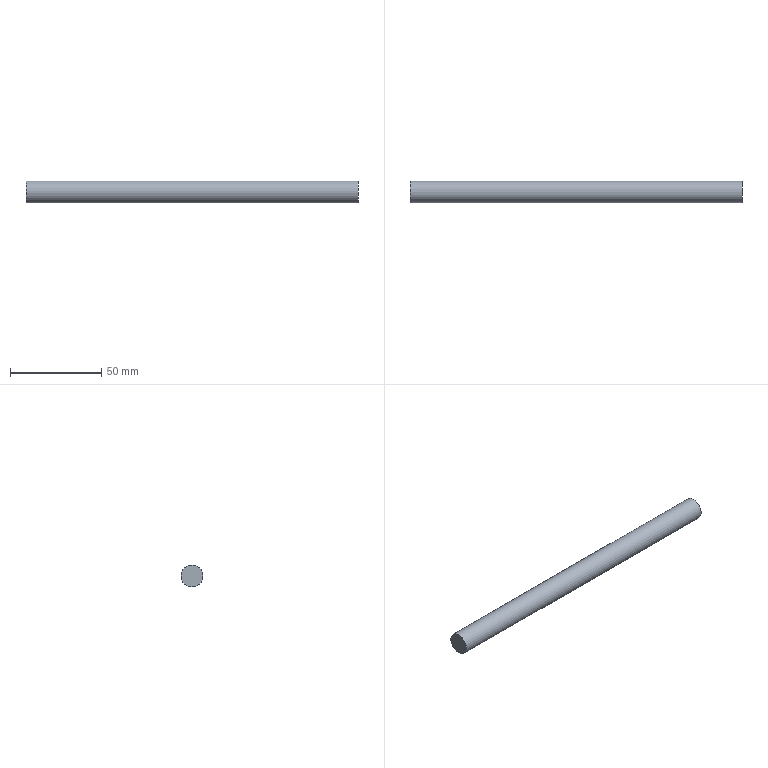Part | STEP file | solid 111 | 1 solid | 3 faces | box 182 x 12 x 12 mm | volume 20584 mm3 | plane 2 | cylinder 1 | commonest cylinder face diameters 12 x1